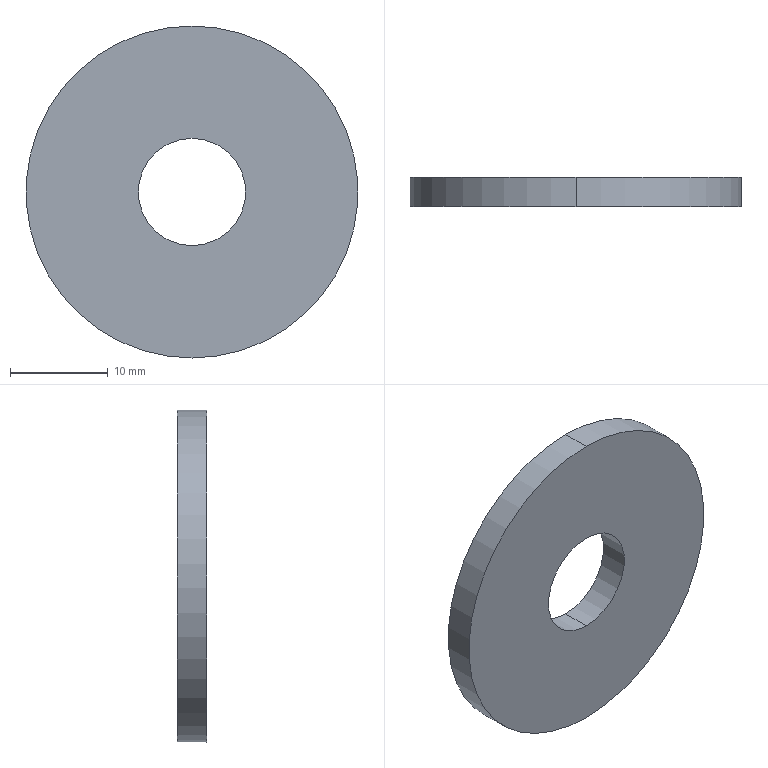Part | SolidWorks | features Revolution 1 | 1 solid | 6 faces | box 34 x 3 x 34 mm | volume 2439 mm3 | cylinder 4 | plane 2 | commonest cylinder face diameters 11 x2 34 x2
STEP:
#1=CARTESIAN_POINT('',(0.,11.645,-17.));
#2=VERTEX_POINT('',#1);
#3=CARTESIAN_POINT('',(0.,11.645,17.));
#4=VERTEX_POINT('',#3);
#5=CARTESIAN_POINT('',(0.,11.645,0.));
#6=DIRECTION('',(0.,-1.,0.));
#7=DIRECTION('',(0.,0.,-1.));
#8=AXIS2_PLACEMENT_3D('',#5,#6,#7);
#9=CIRCLE('',#8,17.);
#10=EDGE_CURVE('',#2,#4,#9,.T.);
#11=ORIENTED_EDGE('',*,*,#10,.T.);
#12=CARTESIAN_POINT('',(0.,8.645,17.));
#13=VERTEX_POINT('',#12);
#14=CARTESIAN_POINT('',(0.,0.,17.));
#15=DIRECTION('',(0.,-1.,0.));
#16=VECTOR('',#15,1000.);
#17=LINE('',#14,#16);
#18=EDGE_CURVE('',#4,#13,#17,.T.);
#19=ORIENTED_EDGE('',*,*,#18,.T.);
#20=CARTESIAN_POINT('',(0.,8.645,-17.));
#21=VERTEX_POINT('',#20);
#22=CARTESIAN_POINT('',(0.,8.645,0.));
#23=DIRECTION('',(0.,-1.,0.));
#24=DIRECTION('',(0.,0.,-1.));
#25=AXIS2_PLACEMENT_3D('',#22,#23,#24);
#26=CIRCLE('',#25,17.);
#27=EDGE_CURVE('',#21,#13,#26,.T.);
#28=ORIENTED_EDGE('',*,*,#27,.F.);
#29=CARTESIAN_POINT('',(0.,0.,-17.));
#30=DIRECTION('',(0.,-1.,0.));
#31=VECTOR('',#30,1000.);
#32=LINE('',#29,#31);
#33=EDGE_CURVE('',#2,#21,#32,.T.);
#34=ORIENTED_EDGE('',*,*,#33,.F.);
#35=EDGE_LOOP('',(#11,#19,#28,#34));
#36=FACE_OUTER_BOUND('',#35,.T.);
#37=CARTESIAN_POINT('',(0.,0.,0.));
#38=DIRECTION('',(0.,-1.,0.));
#39=DIRECTION('',(0.,0.,-1.));
#40=AXIS2_PLACEMENT_3D('',#37,#38,#39);
#41=CYLINDRICAL_SURFACE('',#40,17.);
#42=ADVANCED_FACE('',(#36),#41,.T.);
#43=CARTESIAN_POINT('',(0.,11.645,5.5));
#44=VERTEX_POINT('',#43);
#45=CARTESIAN_POINT('',(0.,11.645,-5.5));
#46=VERTEX_POINT('',#45);
#47=CARTESIAN_POINT('',(0.,11.645,0.));
#48=DIRECTION('',(0.,-1.,0.));
#49=DIRECTION('',(0.,0.,-1.));
#50=AXIS2_PLACEMENT_3D('',#47,#48,#49);
#51=CIRCLE('',#50,5.5);
#52=EDGE_CURVE('',#44,#46,#51,.T.);
#53=ORIENTED_EDGE('',*,*,#52,.F.);
#54=CARTESIAN_POINT('',(0.,8.645,5.5));
#55=VERTEX_POINT('',#54);
#56=CARTESIAN_POINT('',(0.,0.,5.5));
#57=DIRECTION('',(0.,-1.,0.));
#58=VECTOR('',#57,1000.);
#59=LINE('',#56,#58);
#60=EDGE_CURVE('',#44,#55,#59,.T.);
#61=ORIENTED_EDGE('',*,*,#60,.T.);
#62=CARTESIAN_POINT('',(0.,8.645,-5.5));
#63=VERTEX_POINT('',#62);
#64=CARTESIAN_POINT('',(0.,8.645,0.));
#65=DIRECTION('',(0.,-1.,0.));
#66=DIRECTION('',(0.,0.,-1.));
#67=AXIS2_PLACEMENT_3D('',#64,#65,#66);
#68=CIRCLE('',#67,5.5);
#69=EDGE_CURVE('',#55,#63,#68,.T.);
#70=ORIENTED_EDGE('',*,*,#69,.T.);
#71=CARTESIAN_POINT('',(0.,0.,-5.5));
#72=DIRECTION('',(0.,-1.,0.));
#73=VECTOR('',#72,1000.);
#74=LINE('',#71,#73);
#75=EDGE_CURVE('',#46,#63,#74,.T.);
#76=ORIENTED_EDGE('',*,*,#75,.F.);
#77=EDGE_LOOP('',(#53,#61,#70,#76));
#78=FACE_OUTER_BOUND('',#77,.T.);
#79=CARTESIAN_POINT('',(0.,0.,0.));
#80=DIRECTION('',(0.,-1.,0.));
#81=DIRECTION('',(0.,0.,-1.));
#82=AXIS2_PLACEMENT_3D('',#79,#80,#81);
#83=CYLINDRICAL_SURFACE('',#82,5.5);
#84=ADVANCED_FACE('',(#78),#83,.F.);
#85=ORIENTED_EDGE('',*,*,#60,.F.);
#86=CARTESIAN_POINT('',(0.,11.645,0.));
#87=DIRECTION('',(0.,-1.,0.));
#88=DIRECTION('',(0.,0.,-1.));
#89=AXIS2_PLACEMENT_3D('',#86,#87,#88);
#90=CIRCLE('',#89,5.5);
#91=EDGE_CURVE('',#46,#44,#90,.T.);
#92=ORIENTED_EDGE('',*,*,#91,.F.);
#93=ORIENTED_EDGE('',*,*,#75,.T.);
#94=CARTESIAN_POINT('',(0.,8.645,0.));
#95=DIRECTION('',(0.,-1.,0.));
#96=DIRECTION('',(0.,0.,-1.));
#97=AXIS2_PLACEMENT_3D('',#94,#95,#96);
#98=CIRCLE('',#97,5.5);
#99=EDGE_CURVE('',#63,#55,#98,.T.);
#100=ORIENTED_EDGE('',*,*,#99,.T.);
#101=EDGE_LOOP('',(#85,#92,#93,#100));
#102=FACE_OUTER_BOUND('',#101,.T.);
#103=CARTESIAN_POINT('',(0.,0.,0.));
#104=DIRECTION('',(0.,-1.,0.));
#105=DIRECTION('',(0.,0.,-1.));
#106=AXIS2_PLACEMENT_3D('',#103,#104,#105);
#107=CYLINDRICAL_SURFACE('',#106,5.5);
#108=ADVANCED_FACE('',(#102),#107,.F.);
#109=ORIENTED_EDGE('',*,*,#10,.F.);
#110=CARTESIAN_POINT('',(0.,11.645,0.));
#111=DIRECTION('',(0.,-1.,0.));
#112=DIRECTION('',(0.,0.,-1.));
#113=AXIS2_PLACEMENT_3D('',#110,#111,#112);
#114=CIRCLE('',#113,17.);
#115=EDGE_CURVE('',#4,#2,#114,.T.);
#116=ORIENTED_EDGE('',*,*,#115,.F.);
#117=EDGE_LOOP('',(#109,#116));
#118=FACE_OUTER_BOUND('',#117,.T.);
#119=ORIENTED_EDGE('',*,*,#91,.T.);
#120=ORIENTED_EDGE('',*,*,#52,.T.);
#121=EDGE_LOOP('',(#119,#120));
#122=FACE_BOUND('',#121,.T.);
#123=CARTESIAN_POINT('',(-5.5,11.645,0.));
#124=DIRECTION('',(0.,-1.,0.));
#125=DIRECTION('',(0.,0.,-1.));
#126=AXIS2_PLACEMENT_3D('',#123,#124,#125);
#127=PLANE('',#126);
#128=ADVANCED_FACE('',(#118,#122),#127,.F.);
#129=ORIENTED_EDGE('',*,*,#18,.F.);
#130=ORIENTED_EDGE('',*,*,#115,.T.);
#131=ORIENTED_EDGE('',*,*,#33,.T.);
#132=CARTESIAN_POINT('',(0.,8.645,0.));
#133=DIRECTION('',(0.,-1.,0.));
#134=DIRECTION('',(0.,0.,-1.));
#135=AXIS2_PLACEMENT_3D('',#132,#133,#134);
#136=CIRCLE('',#135,17.);
#137=EDGE_CURVE('',#13,#21,#136,.T.);
#138=ORIENTED_EDGE('',*,*,#137,.F.);
#139=EDGE_LOOP('',(#129,#130,#131,#138));
#140=FACE_OUTER_BOUND('',#139,.T.);
#141=CARTESIAN_POINT('',(0.,0.,0.));
#142=DIRECTION('',(0.,-1.,0.));
#143=DIRECTION('',(0.,0.,-1.));
#144=AXIS2_PLACEMENT_3D('',#141,#142,#143);
#145=CYLINDRICAL_SURFACE('',#144,17.);
#146=ADVANCED_FACE('',(#140),#145,.T.);
#147=ORIENTED_EDGE('',*,*,#99,.F.);
#148=ORIENTED_EDGE('',*,*,#69,.F.);
#149=EDGE_LOOP('',(#147,#148));
#150=FACE_BOUND('',#149,.T.);
#151=ORIENTED_EDGE('',*,*,#27,.T.);
#152=ORIENTED_EDGE('',*,*,#137,.T.);
#153=EDGE_LOOP('',(#151,#152));
#154=FACE_OUTER_BOUND('',#153,.T.);
#155=CARTESIAN_POINT('',(-5.5,8.645,0.));
#156=DIRECTION('',(0.,1.,0.));
#157=DIRECTION('',(0.,0.,1.));
#158=AXIS2_PLACEMENT_3D('',#155,#156,#157);
#159=PLANE('',#158);
#160=ADVANCED_FACE('',(#150,#154),#159,.F.);
#161=CLOSED_SHELL('',(#42,#84,#108,#128,#146,#160));
#162=MANIFOLD_SOLID_BREP('',#161);
#163=CARTESIAN_POINT('',(0.,0.,0.));
#164=DIRECTION('',(0.,0.,1.));
#165=DIRECTION('',(1.,0.,0.));
#166=AXIS2_PLACEMENT_3D('',#163,#164,#165);
#167=(LENGTH_UNIT()NAMED_UNIT(*)SI_UNIT(.MILLI.,.METRE.));
#168=UNCERTAINTY_MEASURE_WITH_UNIT(LENGTH_MEASURE(0.00001),#167,'','');
#169=(NAMED_UNIT(*)PLANE_ANGLE_UNIT()SI_UNIT($,.RADIAN.));
#170=(NAMED_UNIT(*)SI_UNIT($,.STERADIAN.)SOLID_ANGLE_UNIT());
#171=(GEOMETRIC_REPRESENTATION_CONTEXT(3)GLOBAL_UNCERTAINTY_ASSIGNED_CONTEXT((#168))GLOBAL_UNIT_ASSIGNED_CONTEXT((#167,#169,#170))REPRESENTATION_CONTEXT('',''));
#172=ADVANCED_BREP_SHAPE_REPRESENTATION('',(#162,#166),#171);